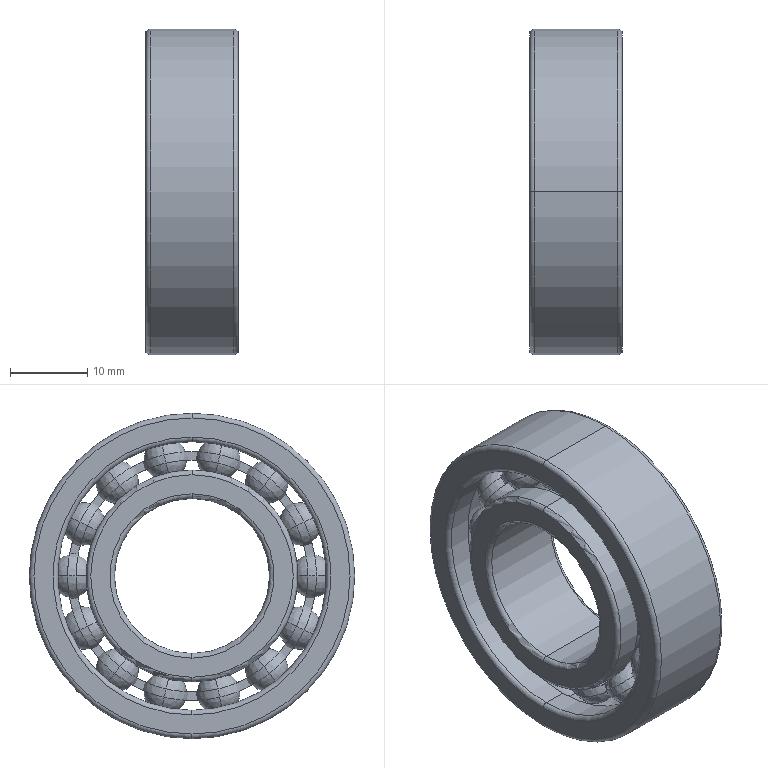Part | SolidWorks | features Revolution 4, CirPattern 2, RefAxis 1, RevCut 1 | 16 solids | 180 faces | box 12 x 42 x 42 mm | volume 9401 mm3 | cylinder 66 | sphere 60 | plane 32 | torus 22 | commonest cylinder face diameters 29.9 x27 32.1 x27 27.333 x4 34.667 x4 20 x2 42 x2